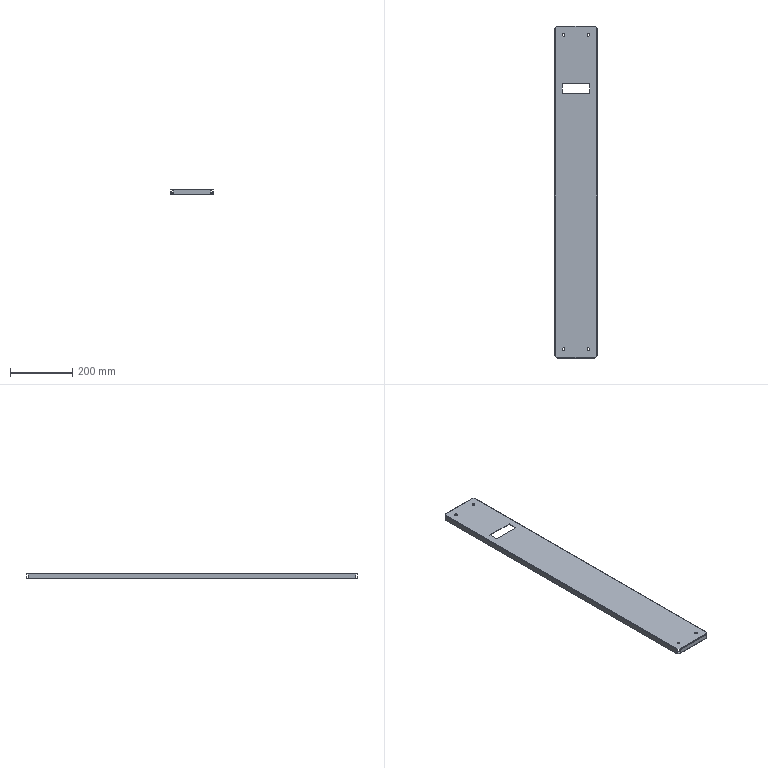Part | SolidWorks | features BaseBody 1 | 1 solid | 50 faces | box 136 x 1066 x 18 mm | volume 272590 mm3 | plane 30 | cylinder 20 | commonest cylinder face diameters 9 x8 1.473 x6 4.473 x6